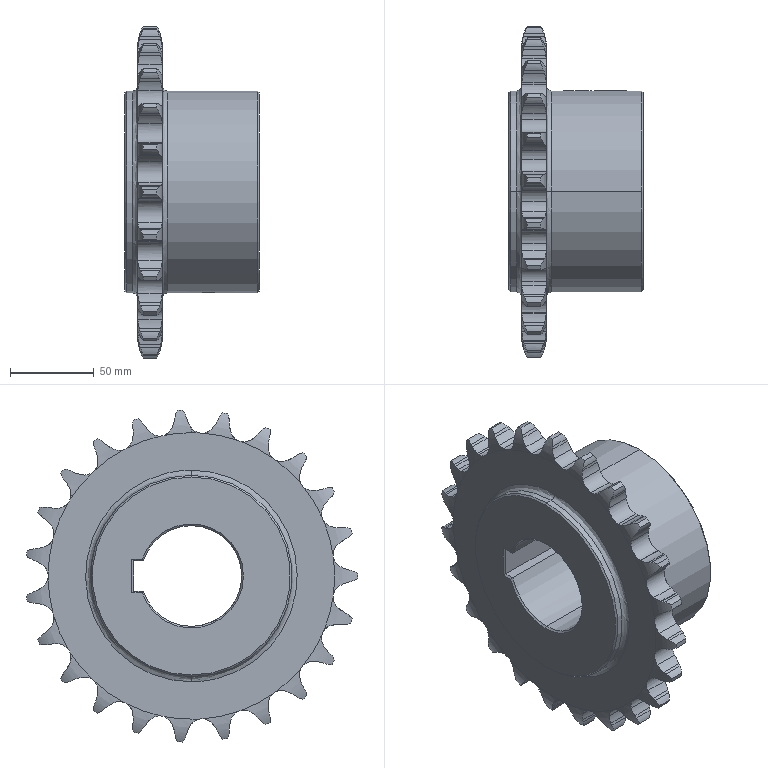Part | STEP file | 1 solid | 281 faces | box 80 x 197.271 x 197.721 mm | volume 875522 mm3 | cylinder 161 | plane 59 | spline 52 | cone 9 | commonest cylinder face diameters 23.032 x49 41.467 x48 16.059 x30 198 x23 10.2 x4 120 x4